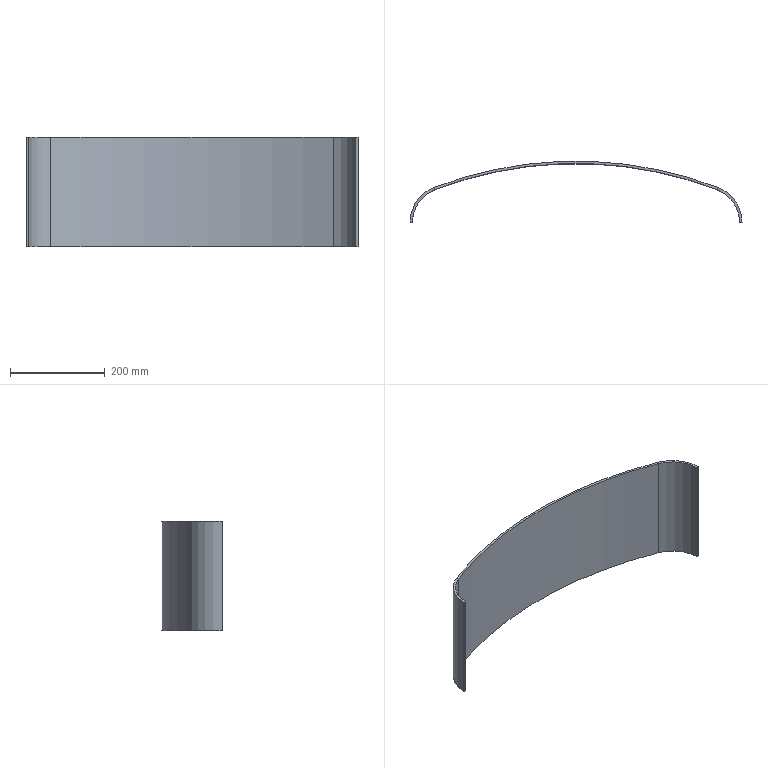Part | SolidWorks | features FlatPattern 1, ICE 1, SMBaseFlange 1, SheetMetal 1 | 1 solid | 16 faces | box 700.002 x 128.973 x 230 mm | volume 913627 mm3 | cylinder 8 | plane 8 | commonest cylinder face diameters 146.078 x3 156.078 x3 1660 x1 1670 x1
STEP:
#1=CARTESIAN_POINT('',(101.796,68.58,230.));
#2=VERTEX_POINT('',#1);
#3=CARTESIAN_POINT('',(54.999,0.418,230.));
#4=VERTEX_POINT('',#3);
#5=CARTESIAN_POINT('',(128.038,0.418,230.));
#6=DIRECTION('',(0.,0.,1.));
#7=DIRECTION('',(1.,0.,0.));
#8=AXIS2_PLACEMENT_3D('',#5,#6,#7);
#9=CIRCLE('',#8,73.039);
#10=EDGE_CURVE('',#2,#4,#9,.T.);
#11=ORIENTED_EDGE('',*,*,#10,.T.);
#12=CARTESIAN_POINT('',(54.999,0.418,0.));
#13=VERTEX_POINT('',#12);
#14=CARTESIAN_POINT('',(54.999,0.418,230.));
#15=DIRECTION('',(0.,0.,-1.));
#16=VECTOR('',#15,1000.);
#17=LINE('',#14,#16);
#18=EDGE_CURVE('',#4,#13,#17,.T.);
#19=ORIENTED_EDGE('',*,*,#18,.T.);
#20=CARTESIAN_POINT('',(101.796,68.58,0.));
#21=VERTEX_POINT('',#20);
#22=CARTESIAN_POINT('',(128.038,0.418,0.));
#23=DIRECTION('',(0.,0.,1.));
#24=DIRECTION('',(1.,0.,0.));
#25=AXIS2_PLACEMENT_3D('',#22,#23,#24);
#26=CIRCLE('',#25,73.039);
#27=EDGE_CURVE('',#21,#13,#26,.T.);
#28=ORIENTED_EDGE('',*,*,#27,.F.);
#29=CARTESIAN_POINT('',(101.796,68.58,230.));
#30=DIRECTION('',(0.,0.,-1.));
#31=VECTOR('',#30,1000.);
#32=LINE('',#29,#31);
#33=EDGE_CURVE('',#2,#21,#32,.T.);
#34=ORIENTED_EDGE('',*,*,#33,.F.);
#35=EDGE_LOOP('',(#11,#19,#28,#34));
#36=FACE_OUTER_BOUND('',#35,.T.);
#37=CARTESIAN_POINT('',(128.038,0.418,230.));
#38=DIRECTION('',(0.,0.,-1.));
#39=DIRECTION('',(-1.,0.,0.));
#40=AXIS2_PLACEMENT_3D('',#37,#38,#39);
#41=CYLINDRICAL_SURFACE('',#40,73.039);
#42=ADVANCED_FACE('',(#36),#41,.F.);
#43=CARTESIAN_POINT('',(49.999,0.418,230.));
#44=VERTEX_POINT('',#43);
#45=CARTESIAN_POINT('',(50.,0.02678,230.));
#46=VERTEX_POINT('',#45);
#47=CARTESIAN_POINT('',(128.038,0.418,230.));
#48=DIRECTION('',(0.,0.,1.));
#49=DIRECTION('',(1.,0.,0.));
#50=AXIS2_PLACEMENT_3D('',#47,#48,#49);
#51=CIRCLE('',#50,78.039);
#52=EDGE_CURVE('',#44,#46,#51,.T.);
#53=ORIENTED_EDGE('',*,*,#52,.F.);
#54=CARTESIAN_POINT('',(49.999,0.418,0.));
#55=VERTEX_POINT('',#54);
#56=CARTESIAN_POINT('',(49.999,0.418,230.));
#57=DIRECTION('',(0.,0.,-1.));
#58=VECTOR('',#57,1000.);
#59=LINE('',#56,#58);
#60=EDGE_CURVE('',#44,#55,#59,.T.);
#61=ORIENTED_EDGE('',*,*,#60,.T.);
#62=CARTESIAN_POINT('',(50.,0.02678,0.));
#63=VERTEX_POINT('',#62);
#64=CARTESIAN_POINT('',(128.038,0.418,0.));
#65=DIRECTION('',(0.,0.,1.));
#66=DIRECTION('',(1.,0.,0.));
#67=AXIS2_PLACEMENT_3D('',#64,#65,#66);
#68=CIRCLE('',#67,78.039);
#69=EDGE_CURVE('',#55,#63,#68,.T.);
#70=ORIENTED_EDGE('',*,*,#69,.T.);
#71=CARTESIAN_POINT('',(50.,0.02678,230.));
#72=DIRECTION('',(0.,0.,1.));
#73=VECTOR('',#72,1000.);
#74=LINE('',#71,#73);
#75=EDGE_CURVE('',#63,#46,#74,.T.);
#76=ORIENTED_EDGE('',*,*,#75,.T.);
#77=EDGE_LOOP('',(#53,#61,#70,#76));
#78=FACE_OUTER_BOUND('',#77,.T.);
#79=CARTESIAN_POINT('',(128.038,0.418,230.));
#80=DIRECTION('',(0.,0.,-1.));
#81=DIRECTION('',(-1.,0.,0.));
#82=AXIS2_PLACEMENT_3D('',#79,#80,#81);
#83=CYLINDRICAL_SURFACE('',#82,78.039);
#84=ADVANCED_FACE('',(#78),#83,.T.);
#85=CARTESIAN_POINT('',(100.,73.246,230.));
#86=VERTEX_POINT('',#85);
#87=CARTESIAN_POINT('',(101.796,68.58,230.));
#88=DIRECTION('',(-0.3593,0.9332,0.));
#89=VECTOR('',#88,1000.);
#90=LINE('',#87,#89);
#91=EDGE_CURVE('',#2,#86,#90,.T.);
#92=ORIENTED_EDGE('',*,*,#91,.F.);
#93=CARTESIAN_POINT('',(698.204,68.58,230.));
#94=VERTEX_POINT('',#93);
#95=CARTESIAN_POINT('',(400.,-706.,230.));
#96=DIRECTION('',(0.,0.,1.));
#97=DIRECTION('',(1.,0.,0.));
#98=AXIS2_PLACEMENT_3D('',#95,#96,#97);
#99=CIRCLE('',#98,830.);
#100=EDGE_CURVE('',#94,#2,#99,.T.);
#101=ORIENTED_EDGE('',*,*,#100,.F.);
#102=CARTESIAN_POINT('',(700.,73.246,230.));
#103=VERTEX_POINT('',#102);
#104=CARTESIAN_POINT('',(698.204,68.58,230.));
#105=DIRECTION('',(0.3593,0.9332,0.));
#106=VECTOR('',#105,1000.);
#107=LINE('',#104,#106);
#108=EDGE_CURVE('',#94,#103,#107,.T.);
#109=ORIENTED_EDGE('',*,*,#108,.T.);
#110=CARTESIAN_POINT('',(400.,-706.,230.));
#111=DIRECTION('',(0.,0.,1.));
#112=DIRECTION('',(-1.,0.,0.));
#113=AXIS2_PLACEMENT_3D('',#110,#111,#112);
#114=CIRCLE('',#113,835.);
#115=EDGE_CURVE('',#103,#86,#114,.T.);
#116=ORIENTED_EDGE('',*,*,#115,.T.);
#117=EDGE_LOOP('',(#92,#101,#109,#116));
#118=FACE_OUTER_BOUND('',#117,.T.);
#119=CARTESIAN_POINT('',(101.796,68.58,230.));
#120=DIRECTION('',(0.,0.,1.));
#121=DIRECTION('',(1.,0.,0.));
#122=AXIS2_PLACEMENT_3D('',#119,#120,#121);
#123=PLANE('',#122);
#124=ADVANCED_FACE('',(#118),#123,.T.);
#125=CARTESIAN_POINT('',(100.,73.246,0.));
#126=VERTEX_POINT('',#125);
#127=CARTESIAN_POINT('',(100.,73.246,0.));
#128=DIRECTION('',(0.3593,-0.9332,0.));
#129=VECTOR('',#128,1000.);
#130=LINE('',#127,#129);
#131=EDGE_CURVE('',#126,#21,#130,.T.);
#132=ORIENTED_EDGE('',*,*,#131,.F.);
#133=CARTESIAN_POINT('',(700.,73.246,0.));
#134=VERTEX_POINT('',#133);
#135=CARTESIAN_POINT('',(400.,-706.,0.));
#136=DIRECTION('',(0.,0.,1.));
#137=DIRECTION('',(-1.,0.,0.));
#138=AXIS2_PLACEMENT_3D('',#135,#136,#137);
#139=CIRCLE('',#138,835.);
#140=EDGE_CURVE('',#134,#126,#139,.T.);
#141=ORIENTED_EDGE('',*,*,#140,.F.);
#142=CARTESIAN_POINT('',(698.204,68.58,0.));
#143=VERTEX_POINT('',#142);
#144=CARTESIAN_POINT('',(700.,73.246,0.));
#145=DIRECTION('',(-0.3593,-0.9332,0.));
#146=VECTOR('',#145,1000.);
#147=LINE('',#144,#146);
#148=EDGE_CURVE('',#134,#143,#147,.T.);
#149=ORIENTED_EDGE('',*,*,#148,.T.);
#150=CARTESIAN_POINT('',(400.,-706.,0.));
#151=DIRECTION('',(0.,0.,1.));
#152=DIRECTION('',(1.,0.,0.));
#153=AXIS2_PLACEMENT_3D('',#150,#151,#152);
#154=CIRCLE('',#153,830.);
#155=EDGE_CURVE('',#143,#21,#154,.T.);
#156=ORIENTED_EDGE('',*,*,#155,.T.);
#157=EDGE_LOOP('',(#132,#141,#149,#156));
#158=FACE_OUTER_BOUND('',#157,.T.);
#159=CARTESIAN_POINT('',(100.,73.246,0.));
#160=DIRECTION('',(0.,0.,-1.));
#161=DIRECTION('',(-1.,0.,0.));
#162=AXIS2_PLACEMENT_3D('',#159,#160,#161);
#163=PLANE('',#162);
#164=ADVANCED_FACE('',(#158),#163,.T.);
#165=CARTESIAN_POINT('',(750.,0.02678,230.));
#166=VERTEX_POINT('',#165);
#167=CARTESIAN_POINT('',(745.,0.02678,230.));
#168=VERTEX_POINT('',#167);
#169=CARTESIAN_POINT('',(49.846,0.02678,230.));
#170=DIRECTION('',(-1.,0.,0.));
#171=VECTOR('',#170,1000.);
#172=LINE('',#169,#171);
#173=EDGE_CURVE('',#166,#168,#172,.T.);
#174=ORIENTED_EDGE('',*,*,#173,.F.);
#175=CARTESIAN_POINT('',(671.962,0.418,230.));
#176=DIRECTION('',(0.,0.,1.));
#177=DIRECTION('',(-1.,0.,0.));
#178=AXIS2_PLACEMENT_3D('',#175,#176,#177);
#179=CIRCLE('',#178,78.039);
#180=EDGE_CURVE('',#166,#103,#179,.T.);
#181=ORIENTED_EDGE('',*,*,#180,.T.);
#182=ORIENTED_EDGE('',*,*,#108,.F.);
#183=CARTESIAN_POINT('',(671.962,0.418,230.));
#184=DIRECTION('',(0.,0.,1.));
#185=DIRECTION('',(1.,0.,0.));
#186=AXIS2_PLACEMENT_3D('',#183,#184,#185);
#187=CIRCLE('',#186,73.039);
#188=EDGE_CURVE('',#168,#94,#187,.T.);
#189=ORIENTED_EDGE('',*,*,#188,.F.);
#190=EDGE_LOOP('',(#174,#181,#182,#189));
#191=FACE_OUTER_BOUND('',#190,.T.);
#192=CARTESIAN_POINT('',(698.204,68.58,230.));
#193=DIRECTION('',(0.,0.,1.));
#194=DIRECTION('',(1.,0.,0.));
#195=AXIS2_PLACEMENT_3D('',#192,#193,#194);
#196=PLANE('',#195);
#197=ADVANCED_FACE('',(#191),#196,.T.);
#198=CARTESIAN_POINT('',(750.,0.02678,0.));
#199=VERTEX_POINT('',#198);
#200=CARTESIAN_POINT('',(745.,0.02678,0.));
#201=VERTEX_POINT('',#200);
#202=CARTESIAN_POINT('',(49.846,0.02678,0.));
#203=DIRECTION('',(-1.,0.,0.));
#204=VECTOR('',#203,1000.);
#205=LINE('',#202,#204);
#206=EDGE_CURVE('',#199,#201,#205,.T.);
#207=ORIENTED_EDGE('',*,*,#206,.T.);
#208=CARTESIAN_POINT('',(671.962,0.418,0.));
#209=DIRECTION('',(0.,0.,1.));
#210=DIRECTION('',(1.,0.,0.));
#211=AXIS2_PLACEMENT_3D('',#208,#209,#210);
#212=CIRCLE('',#211,73.039);
#213=EDGE_CURVE('',#201,#143,#212,.T.);
#214=ORIENTED_EDGE('',*,*,#213,.T.);
#215=ORIENTED_EDGE('',*,*,#148,.F.);
#216=CARTESIAN_POINT('',(671.962,0.418,0.));
#217=DIRECTION('',(0.,0.,1.));
#218=DIRECTION('',(-1.,0.,0.));
#219=AXIS2_PLACEMENT_3D('',#216,#217,#218);
#220=CIRCLE('',#219,78.039);
#221=EDGE_CURVE('',#199,#134,#220,.T.);
#222=ORIENTED_EDGE('',*,*,#221,.F.);
#223=EDGE_LOOP('',(#207,#214,#215,#222));
#224=FACE_OUTER_BOUND('',#223,.T.);
#225=CARTESIAN_POINT('',(700.,73.246,0.));
#226=DIRECTION('',(0.,0.,-1.));
#227=DIRECTION('',(-1.,0.,0.));
#228=AXIS2_PLACEMENT_3D('',#225,#226,#227);
#229=PLANE('',#228);
#230=ADVANCED_FACE('',(#224),#229,.T.);
#231=ORIENTED_EDGE('',*,*,#60,.F.);
#232=CARTESIAN_POINT('',(128.038,0.418,230.));
#233=DIRECTION('',(0.,0.,1.));
#234=DIRECTION('',(1.,0.,0.));
#235=AXIS2_PLACEMENT_3D('',#232,#233,#234);
#236=CIRCLE('',#235,78.039);
#237=EDGE_CURVE('',#86,#44,#236,.T.);
#238=ORIENTED_EDGE('',*,*,#237,.F.);
#239=CARTESIAN_POINT('',(100.,73.246,230.));
#240=DIRECTION('',(0.,0.,-1.));
#241=VECTOR('',#240,1000.);
#242=LINE('',#239,#241);
#243=EDGE_CURVE('',#86,#126,#242,.T.);
#244=ORIENTED_EDGE('',*,*,#243,.T.);
#245=CARTESIAN_POINT('',(128.038,0.418,0.));
#246=DIRECTION('',(0.,0.,1.));
#247=DIRECTION('',(1.,0.,0.));
#248=AXIS2_PLACEMENT_3D('',#245,#246,#247);
#249=CIRCLE('',#248,78.039);
#250=EDGE_CURVE('',#126,#55,#249,.T.);
#251=ORIENTED_EDGE('',*,*,#250,.T.);
#252=EDGE_LOOP('',(#231,#238,#244,#251));
#253=FACE_OUTER_BOUND('',#252,.T.);
#254=CARTESIAN_POINT('',(128.038,0.418,230.));
#255=DIRECTION('',(0.,0.,-1.));
#256=DIRECTION('',(-1.,0.,0.));
#257=AXIS2_PLACEMENT_3D('',#254,#255,#256);
#258=CYLINDRICAL_SURFACE('',#257,78.039);
#259=ADVANCED_FACE('',(#253),#258,.T.);
#260=ORIENTED_EDGE('',*,*,#18,.F.);
#261=CARTESIAN_POINT('',(55.,0.02678,230.));
#262=VERTEX_POINT('',#261);
#263=CARTESIAN_POINT('',(128.038,0.418,230.));
#264=DIRECTION('',(0.,0.,1.));
#265=DIRECTION('',(1.,0.,0.));
#266=AXIS2_PLACEMENT_3D('',#263,#264,#265);
#267=CIRCLE('',#266,73.039);
#268=EDGE_CURVE('',#4,#262,#267,.T.);
#269=ORIENTED_EDGE('',*,*,#268,.T.);
#270=CARTESIAN_POINT('',(55.,0.02678,0.));
#271=VERTEX_POINT('',#270);
#272=CARTESIAN_POINT('',(55.,0.02678,230.));
#273=DIRECTION('',(0.,0.,-1.));
#274=VECTOR('',#273,1000.);
#275=LINE('',#272,#274);
#276=EDGE_CURVE('',#262,#271,#275,.T.);
#277=ORIENTED_EDGE('',*,*,#276,.T.);
#278=CARTESIAN_POINT('',(128.038,0.418,0.));
#279=DIRECTION('',(0.,0.,1.));
#280=DIRECTION('',(1.,0.,0.));
#281=AXIS2_PLACEMENT_3D('',#278,#279,#280);
#282=CIRCLE('',#281,73.039);
#283=EDGE_CURVE('',#13,#271,#282,.T.);
#284=ORIENTED_EDGE('',*,*,#283,.F.);
#285=EDGE_LOOP('',(#260,#269,#277,#284));
#286=FACE_OUTER_BOUND('',#285,.T.);
#287=CARTESIAN_POINT('',(128.038,0.418,230.));
#288=DIRECTION('',(0.,0.,-1.));
#289=DIRECTION('',(-1.,0.,0.));
#290=AXIS2_PLACEMENT_3D('',#287,#288,#289);
#291=CYLINDRICAL_SURFACE('',#290,73.039);
#292=ADVANCED_FACE('',(#286),#291,.F.);
#293=ORIENTED_EDGE('',*,*,#155,.F.);
#294=CARTESIAN_POINT('',(698.204,68.58,230.));
#295=DIRECTION('',(0.,0.,-1.));
#296=VECTOR('',#295,1000.);
#297=LINE('',#294,#296);
#298=EDGE_CURVE('',#94,#143,#297,.T.);
#299=ORIENTED_EDGE('',*,*,#298,.F.);
#300=ORIENTED_EDGE('',*,*,#100,.T.);
#301=ORIENTED_EDGE('',*,*,#33,.T.);
#302=EDGE_LOOP('',(#293,#299,#300,#301));
#303=FACE_OUTER_BOUND('',#302,.T.);
#304=CARTESIAN_POINT('',(400.,-706.,230.));
#305=DIRECTION('',(0.,0.,-1.));
#306=DIRECTION('',(-1.,0.,0.));
#307=AXIS2_PLACEMENT_3D('',#304,#305,#306);
#308=CYLINDRICAL_SURFACE('',#307,830.);
#309=ADVANCED_FACE('',(#303),#308,.F.);
#310=ORIENTED_EDGE('',*,*,#213,.F.);
#311=CARTESIAN_POINT('',(745.,0.02678,230.));
#312=DIRECTION('',(0.,0.,-1.));
#313=VECTOR('',#312,1000.);
#314=LINE('',#311,#313);
#315=EDGE_CURVE('',#168,#201,#314,.T.);
#316=ORIENTED_EDGE('',*,*,#315,.F.);
#317=ORIENTED_EDGE('',*,*,#188,.T.);
#318=ORIENTED_EDGE('',*,*,#298,.T.);
#319=EDGE_LOOP('',(#310,#316,#317,#318));
#320=FACE_OUTER_BOUND('',#319,.T.);
#321=CARTESIAN_POINT('',(671.962,0.418,230.));
#322=DIRECTION('',(0.,0.,-1.));
#323=DIRECTION('',(-1.,0.,0.));
#324=AXIS2_PLACEMENT_3D('',#321,#322,#323);
#325=CYLINDRICAL_SURFACE('',#324,73.039);
#326=ADVANCED_FACE('',(#320),#325,.F.);
#327=ORIENTED_EDGE('',*,*,#180,.F.);
#328=CARTESIAN_POINT('',(750.,0.02678,230.));
#329=DIRECTION('',(0.,0.,-1.));
#330=VECTOR('',#329,1000.);
#331=LINE('',#328,#330);
#332=EDGE_CURVE('',#166,#199,#331,.T.);
#333=ORIENTED_EDGE('',*,*,#332,.T.);
#334=ORIENTED_EDGE('',*,*,#221,.T.);
#335=CARTESIAN_POINT('',(700.,73.246,230.));
#336=DIRECTION('',(0.,0.,-1.));
#337=VECTOR('',#336,1000.);
#338=LINE('',#335,#337);
#339=EDGE_CURVE('',#103,#134,#338,.T.);
#340=ORIENTED_EDGE('',*,*,#339,.F.);
#341=EDGE_LOOP('',(#327,#333,#334,#340));
#342=FACE_OUTER_BOUND('',#341,.T.);
#343=CARTESIAN_POINT('',(671.962,0.418,230.));
#344=DIRECTION('',(0.,0.,-1.));
#345=DIRECTION('',(-1.,0.,0.));
#346=AXIS2_PLACEMENT_3D('',#343,#344,#345);
#347=CYLINDRICAL_SURFACE('',#346,78.039);
#348=ADVANCED_FACE('',(#342),#347,.T.);
#349=ORIENTED_EDGE('',*,*,#140,.T.);
#350=ORIENTED_EDGE('',*,*,#243,.F.);
#351=ORIENTED_EDGE('',*,*,#115,.F.);
#352=ORIENTED_EDGE('',*,*,#339,.T.);
#353=EDGE_LOOP('',(#349,#350,#351,#352));
#354=FACE_OUTER_BOUND('',#353,.T.);
#355=CARTESIAN_POINT('',(400.,-706.,230.));
#356=DIRECTION('',(0.,0.,-1.));
#357=DIRECTION('',(-1.,0.,0.));
#358=AXIS2_PLACEMENT_3D('',#355,#356,#357);
#359=CYLINDRICAL_SURFACE('',#358,835.);
#360=ADVANCED_FACE('',(#354),#359,.T.);
#361=CARTESIAN_POINT('',(49.846,0.02678,230.));
#362=DIRECTION('',(-1.,0.,0.));
#363=VECTOR('',#362,1000.);
#364=LINE('',#361,#363);
#365=EDGE_CURVE('',#262,#46,#364,.T.);
#366=ORIENTED_EDGE('',*,*,#365,.F.);
#367=ORIENTED_EDGE('',*,*,#268,.F.);
#368=ORIENTED_EDGE('',*,*,#10,.F.);
#369=ORIENTED_EDGE('',*,*,#91,.T.);
#370=ORIENTED_EDGE('',*,*,#237,.T.);
#371=ORIENTED_EDGE('',*,*,#52,.T.);
#372=EDGE_LOOP('',(#366,#367,#368,#369,#370,#371));
#373=FACE_OUTER_BOUND('',#372,.T.);
#374=CARTESIAN_POINT('',(128.038,0.418,230.));
#375=DIRECTION('',(0.,0.,1.));
#376=DIRECTION('',(1.,0.,0.));
#377=AXIS2_PLACEMENT_3D('',#374,#375,#376);
#378=PLANE('',#377);
#379=ADVANCED_FACE('',(#373),#378,.T.);
#380=ORIENTED_EDGE('',*,*,#27,.T.);
#381=ORIENTED_EDGE('',*,*,#283,.T.);
#382=CARTESIAN_POINT('',(128.038,0.02678,0.));
#383=DIRECTION('',(-1.,0.,0.));
#384=VECTOR('',#383,1000.);
#385=LINE('',#382,#384);
#386=EDGE_CURVE('',#271,#63,#385,.T.);
#387=ORIENTED_EDGE('',*,*,#386,.T.);
#388=ORIENTED_EDGE('',*,*,#69,.F.);
#389=ORIENTED_EDGE('',*,*,#250,.F.);
#390=ORIENTED_EDGE('',*,*,#131,.T.);
#391=EDGE_LOOP('',(#380,#381,#387,#388,#389,#390));
#392=FACE_OUTER_BOUND('',#391,.T.);
#393=CARTESIAN_POINT('',(128.038,0.418,0.));
#394=DIRECTION('',(0.,0.,1.));
#395=DIRECTION('',(1.,0.,0.));
#396=AXIS2_PLACEMENT_3D('',#393,#394,#395);
#397=PLANE('',#396);
#398=ADVANCED_FACE('',(#392),#397,.F.);
#399=ORIENTED_EDGE('',*,*,#386,.F.);
#400=ORIENTED_EDGE('',*,*,#276,.F.);
#401=ORIENTED_EDGE('',*,*,#365,.T.);
#402=ORIENTED_EDGE('',*,*,#75,.F.);
#403=EDGE_LOOP('',(#399,#400,#401,#402));
#404=FACE_OUTER_BOUND('',#403,.T.);
#405=CARTESIAN_POINT('',(49.846,0.02678,0.));
#406=DIRECTION('',(0.,1.,0.));
#407=DIRECTION('',(0.,0.,1.));
#408=AXIS2_PLACEMENT_3D('',#405,#406,#407);
#409=PLANE('',#408);
#410=ADVANCED_FACE('',(#404),#409,.F.);
#411=ORIENTED_EDGE('',*,*,#315,.T.);
#412=ORIENTED_EDGE('',*,*,#206,.F.);
#413=ORIENTED_EDGE('',*,*,#332,.F.);
#414=ORIENTED_EDGE('',*,*,#173,.T.);
#415=EDGE_LOOP('',(#411,#412,#413,#414));
#416=FACE_OUTER_BOUND('',#415,.T.);
#417=CARTESIAN_POINT('',(49.846,0.02678,0.));
#418=DIRECTION('',(0.,1.,0.));
#419=DIRECTION('',(0.,0.,1.));
#420=AXIS2_PLACEMENT_3D('',#417,#418,#419);
#421=PLANE('',#420);
#422=ADVANCED_FACE('',(#416),#421,.F.);
#423=CLOSED_SHELL('',(#42,#84,#124,#164,#197,#230,#259,#292,#309,#326,#348,#360,#379,#398,#410,#422));
#424=MANIFOLD_SOLID_BREP('',#423);
#425=CARTESIAN_POINT('',(0.,0.,0.));
#426=DIRECTION('',(0.,0.,1.));
#427=DIRECTION('',(1.,0.,0.));
#428=AXIS2_PLACEMENT_3D('',#425,#426,#427);
#429=(LENGTH_UNIT()NAMED_UNIT(*)SI_UNIT(.MILLI.,.METRE.));
#430=UNCERTAINTY_MEASURE_WITH_UNIT(LENGTH_MEASURE(0.00001),#429,'','');
#431=(NAMED_UNIT(*)PLANE_ANGLE_UNIT()SI_UNIT($,.RADIAN.));
#432=(NAMED_UNIT(*)SI_UNIT($,.STERADIAN.)SOLID_ANGLE_UNIT());
#433=(GEOMETRIC_REPRESENTATION_CONTEXT(3)GLOBAL_UNCERTAINTY_ASSIGNED_CONTEXT((#430))GLOBAL_UNIT_ASSIGNED_CONTEXT((#429,#431,#432))REPRESENTATION_CONTEXT('',''));
#434=ADVANCED_BREP_SHAPE_REPRESENTATION('',(#424,#428),#433);